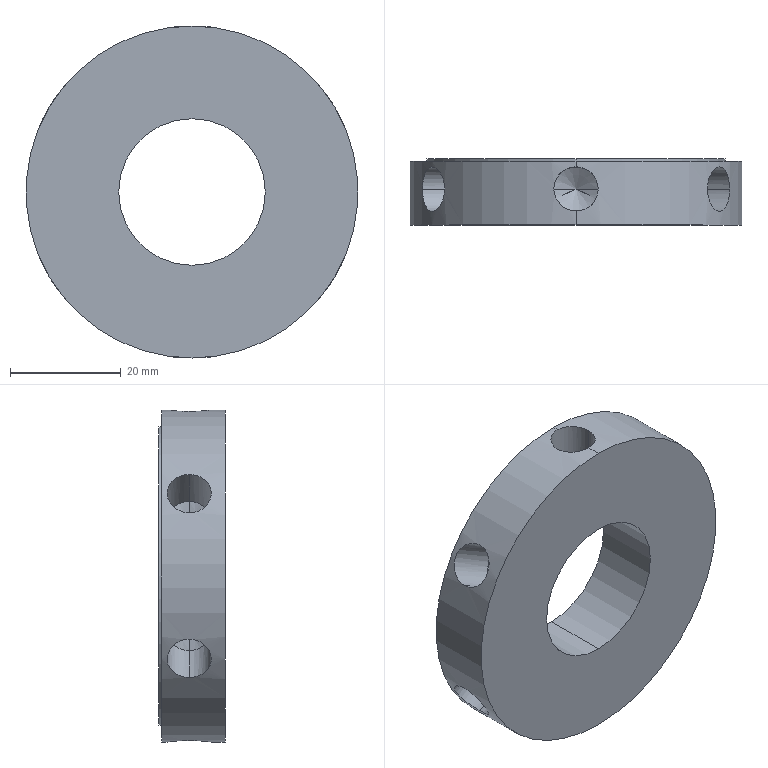Part | STEP file | BU-A14a | 1 solid | 33 faces | box 60 x 12 x 60 mm | volume 23804 mm3 | cylinder 18 | cone 12 | plane 3 | commonest cylinder face diameters 8 x12 26.5 x2 54 x2 60 x2